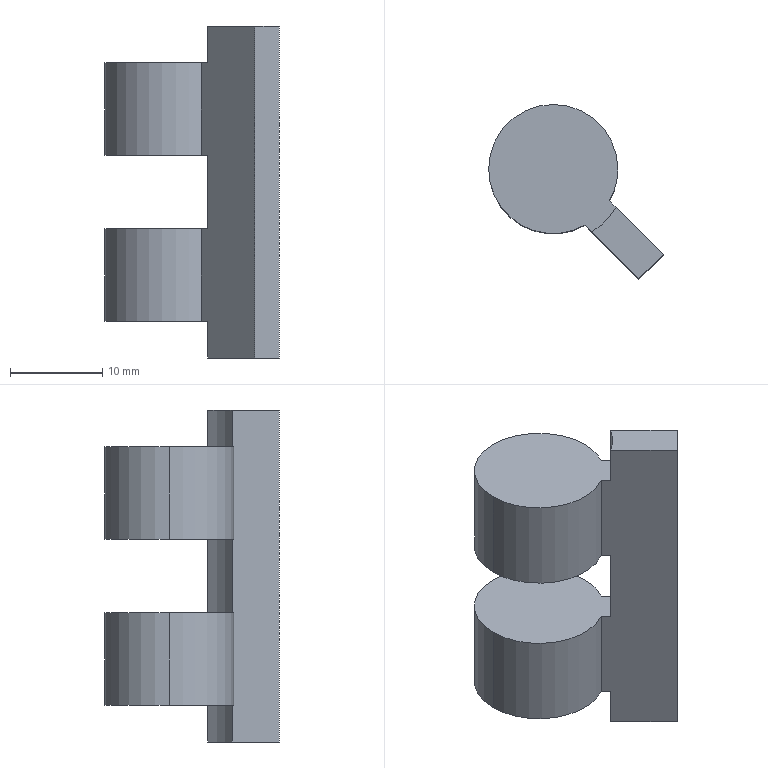Part | STEP file | 1 solid | 18 faces | box 18.932 x 18.932 x 36 mm | volume 4110 mm3 | cylinder 9 | plane 9 | commonest cylinder face diameters 14 x6 16 x3
STEP:
#1=CARTESIAN_POINT('',(0.,0.,0.));
#2=DIRECTION('',(0.,0.,1.));
#3=DIRECTION('',(1.,0.,0.));
#4=AXIS2_PLACEMENT_3D('',#1,#2,#3);
#5=CARTESIAN_POINT('',(-10.892,-5.625,-13.));
#6=VERTEX_POINT('',#5);
#7=CARTESIAN_POINT('',(-10.892,-5.625,-23.));
#8=VERTEX_POINT('',#7);
#9=CARTESIAN_POINT('',(-10.892,-5.625,-13.));
#10=DIRECTION('',(0.,0.,-1.));
#11=VECTOR('',#10,1.);
#12=LINE('',#9,#11);
#13=CARTESIAN_POINT('',(-3.892,-5.625,-23.));
#14=DIRECTION('',(0.,0.,1.));
#15=DIRECTION('',(-1.,0.,0.));
#16=AXIS2_PLACEMENT_3D('',#13,#14,#15);
#17=CYLINDRICAL_SURFACE('',#16,7.);
#18=CARTESIAN_POINT('',(6.283,10.));
#19=DIRECTION('',(0.,-1.));
#20=VECTOR('',#19,1.);
#21=LINE('',#18,#20);
#22=(GEOMETRIC_REPRESENTATION_CONTEXT(2)PARAMETRIC_REPRESENTATION_CONTEXT()REPRESENTATION_CONTEXT('',''));
#23=DEFINITIONAL_REPRESENTATION('',(#21),#22);
#24=PCURVE('',#17,#23);
#25=CARTESIAN_POINT('',(-3.892,-5.625,-23.));
#26=DIRECTION('',(0.,0.,1.));
#27=DIRECTION('',(-1.,0.,0.));
#28=AXIS2_PLACEMENT_3D('',#25,#26,#27);
#29=CYLINDRICAL_SURFACE('',#28,7.);
#30=CARTESIAN_POINT('',(0.,10.));
#31=DIRECTION('',(0.,-1.));
#32=VECTOR('',#31,1.);
#33=LINE('',#30,#32);
#34=(GEOMETRIC_REPRESENTATION_CONTEXT(2)PARAMETRIC_REPRESENTATION_CONTEXT()REPRESENTATION_CONTEXT('',''));
#35=DEFINITIONAL_REPRESENTATION('',(#33),#34);
#36=PCURVE('',#29,#35);
#37=SURFACE_CURVE('',#12,(#24,#36),.PCURVE_S1.);
#38=EDGE_CURVE('',#6,#8,#37,.T.);
#39=ORIENTED_EDGE('',*,*,#38,.F.);
#40=CARTESIAN_POINT('',(3.108,-5.625,-13.));
#41=VERTEX_POINT('',#40);
#42=CARTESIAN_POINT('',(-3.892,-5.625,-13.));
#43=DIRECTION('',(0.,0.,1.));
#44=DIRECTION('',(1.,0.,0.));
#45=AXIS2_PLACEMENT_3D('',#42,#43,#44);
#46=CIRCLE('',#45,7.);
#47=CARTESIAN_POINT('',(3.142,10.));
#48=DIRECTION('',(1.,0.));
#49=VECTOR('',#48,1.);
#50=LINE('',#47,#49);
#51=(GEOMETRIC_REPRESENTATION_CONTEXT(2)PARAMETRIC_REPRESENTATION_CONTEXT()REPRESENTATION_CONTEXT('',''));
#52=DEFINITIONAL_REPRESENTATION('',(#50),#51);
#53=PCURVE('',#17,#52);
#54=CARTESIAN_POINT('',(-3.892,-5.625,-13.));
#55=DIRECTION('',(0.,0.,1.));
#56=DIRECTION('',(-1.,0.,0.));
#57=AXIS2_PLACEMENT_3D('',#54,#55,#56);
#58=PLANE('',#57);
#59=CARTESIAN_POINT('',(0.,0.));
#60=DIRECTION('',(-1.,0.));
#61=AXIS2_PLACEMENT_2D('',#59,#60);
#62=CIRCLE('',#61,7.);
#63=(GEOMETRIC_REPRESENTATION_CONTEXT(2)PARAMETRIC_REPRESENTATION_CONTEXT()REPRESENTATION_CONTEXT('',''));
#64=DEFINITIONAL_REPRESENTATION('',(#62),#63);
#65=PCURVE('',#58,#64);
#66=SURFACE_CURVE('',#46,(#53,#65),.PCURVE_S1.);
#67=EDGE_CURVE('',#41,#6,#66,.T.);
#68=ORIENTED_EDGE('',*,*,#67,.F.);
#69=CARTESIAN_POINT('',(3.108,-5.625,-23.));
#70=VERTEX_POINT('',#69);
#71=CARTESIAN_POINT('',(3.108,-5.625,-13.));
#72=DIRECTION('',(0.,0.,-1.));
#73=VECTOR('',#72,1.);
#74=LINE('',#71,#73);
#75=CARTESIAN_POINT('',(3.142,10.));
#76=DIRECTION('',(0.,-1.));
#77=VECTOR('',#76,1.);
#78=LINE('',#75,#77);
#79=(GEOMETRIC_REPRESENTATION_CONTEXT(2)PARAMETRIC_REPRESENTATION_CONTEXT()REPRESENTATION_CONTEXT('',''));
#80=DEFINITIONAL_REPRESENTATION('',(#78),#79);
#81=PCURVE('',#17,#80);
#82=CARTESIAN_POINT('',(-3.892,-5.625,-23.));
#83=DIRECTION('',(0.,0.,1.));
#84=DIRECTION('',(-1.,0.,0.));
#85=AXIS2_PLACEMENT_3D('',#82,#83,#84);
#86=CYLINDRICAL_SURFACE('',#85,7.);
#87=CARTESIAN_POINT('',(3.142,10.));
#88=DIRECTION('',(0.,-1.));
#89=VECTOR('',#88,1.);
#90=LINE('',#87,#89);
#91=(GEOMETRIC_REPRESENTATION_CONTEXT(2)PARAMETRIC_REPRESENTATION_CONTEXT()REPRESENTATION_CONTEXT('',''));
#92=DEFINITIONAL_REPRESENTATION('',(#90),#91);
#93=PCURVE('',#86,#92);
#94=SURFACE_CURVE('',#74,(#81,#93),.PCURVE_S1.);
#95=EDGE_CURVE('',#41,#70,#94,.T.);
#96=ORIENTED_EDGE('',*,*,#95,.T.);
#97=CARTESIAN_POINT('',(-3.892,-5.625,-23.));
#98=DIRECTION('',(0.,0.,-1.));
#99=DIRECTION('',(-1.,0.,0.));
#100=AXIS2_PLACEMENT_3D('',#97,#98,#99);
#101=CIRCLE('',#100,7.);
#102=CARTESIAN_POINT('',(6.283,0.));
#103=DIRECTION('',(-1.,0.));
#104=VECTOR('',#103,1.);
#105=LINE('',#102,#104);
#106=(GEOMETRIC_REPRESENTATION_CONTEXT(2)PARAMETRIC_REPRESENTATION_CONTEXT()REPRESENTATION_CONTEXT('',''));
#107=DEFINITIONAL_REPRESENTATION('',(#105),#106);
#108=PCURVE('',#17,#107);
#109=CARTESIAN_POINT('',(-3.892,-5.625,-23.));
#110=DIRECTION('',(0.,0.,1.));
#111=DIRECTION('',(-1.,0.,0.));
#112=AXIS2_PLACEMENT_3D('',#109,#110,#111);
#113=PLANE('',#112);
#114=CARTESIAN_POINT('',(7.,0.));
#115=CARTESIAN_POINT('',(7.,-12.124));
#116=CARTESIAN_POINT('',(-3.5,-6.062));
#117=CARTESIAN_POINT('',(-14.,0.));
#118=CARTESIAN_POINT('',(-3.5,6.062));
#119=CARTESIAN_POINT('',(7.,12.124));
#120=CARTESIAN_POINT('',(7.,0.));
#121=(BOUNDED_CURVE()B_SPLINE_CURVE(2,(#114,#115,#116,#117,#118,#119,#120),.UNSPECIFIED.,.T.,.F.)B_SPLINE_CURVE_WITH_KNOTS((1,2,2,2,2,1),(-2.094,0.,2.094,4.189,6.283,8.378),.UNSPECIFIED.)CURVE()GEOMETRIC_REPRESENTATION_ITEM()RATIONAL_B_SPLINE_CURVE((1.,0.5,1.,0.5,1.,0.5,1.))REPRESENTATION_ITEM(''));
#122=(GEOMETRIC_REPRESENTATION_CONTEXT(2)PARAMETRIC_REPRESENTATION_CONTEXT()REPRESENTATION_CONTEXT('',''));
#123=DEFINITIONAL_REPRESENTATION('',(#121),#122);
#124=PCURVE('',#113,#123);
#125=SURFACE_CURVE('',#101,(#108,#124),.PCURVE_S1.);
#126=EDGE_CURVE('',#8,#70,#125,.T.);
#127=ORIENTED_EDGE('',*,*,#126,.F.);
#128=EDGE_LOOP('',(#39,#68,#96,#127));
#129=FACE_BOUND('',#128,.T.);
#130=ADVANCED_FACE('',(#129),#17,.T.);
#131=CARTESIAN_POINT('',(0.2816,-12.45,-23.));
#132=VERTEX_POINT('',#131);
#133=CARTESIAN_POINT('',(-0.4488,-11.72,-23.));
#134=VERTEX_POINT('',#133);
#135=CARTESIAN_POINT('',(0.2816,-12.45,-23.));
#136=DIRECTION('',(-0.7071,0.7071,0.));
#137=VECTOR('',#136,1.);
#138=LINE('',#135,#137);
#139=CARTESIAN_POINT('',(-4.173,6.825));
#140=DIRECTION('',(0.7071,-0.7071));
#141=VECTOR('',#140,1.);
#142=LINE('',#139,#141);
#143=(GEOMETRIC_REPRESENTATION_CONTEXT(2)PARAMETRIC_REPRESENTATION_CONTEXT()REPRESENTATION_CONTEXT('',''));
#144=DEFINITIONAL_REPRESENTATION('',(#142),#143);
#145=PCURVE('',#113,#144);
#146=CARTESIAN_POINT('',(-0.4488,-11.72,5.));
#147=DIRECTION('',(0.7071,0.7071,0.));
#148=DIRECTION('',(0.,0.,1.));
#149=AXIS2_PLACEMENT_3D('',#146,#147,#148);
#150=PLANE('',#149);
#151=CARTESIAN_POINT('',(-28.,1.033));
#152=DIRECTION('',(0.,-1.));
#153=VECTOR('',#152,1.);
#154=LINE('',#151,#153);
#155=(GEOMETRIC_REPRESENTATION_CONTEXT(2)PARAMETRIC_REPRESENTATION_CONTEXT()REPRESENTATION_CONTEXT('',''));
#156=DEFINITIONAL_REPRESENTATION('',(#154),#155);
#157=PCURVE('',#150,#156);
#158=SURFACE_CURVE('',#138,(#145,#157),.PCURVE_S1.);
#159=EDGE_CURVE('',#132,#134,#158,.T.);
#160=ORIENTED_EDGE('',*,*,#159,.F.);
#161=CARTESIAN_POINT('',(2.933,-9.798,-23.));
#162=VERTEX_POINT('',#161);
#163=CARTESIAN_POINT('',(-3.892,-5.625,-23.));
#164=DIRECTION('',(0.,0.,-1.));
#165=DIRECTION('',(0.8531,-0.5217,0.));
#166=AXIS2_PLACEMENT_3D('',#163,#164,#165);
#167=CIRCLE('',#166,8.);
#168=CARTESIAN_POINT('',(-6.825,4.173));
#169=CARTESIAN_POINT('',(0.4035,15.995));
#170=CARTESIAN_POINT('',(7.027,3.824));
#171=CARTESIAN_POINT('',(13.65,-8.347));
#172=CARTESIAN_POINT('',(-0.2018,-7.997));
#173=CARTESIAN_POINT('',(-14.054,-7.648));
#174=CARTESIAN_POINT('',(-6.825,4.173));
#175=(BOUNDED_CURVE()B_SPLINE_CURVE(2,(#168,#169,#170,#171,#172,#173,#174),.UNSPECIFIED.,.T.,.F.)B_SPLINE_CURVE_WITH_KNOTS((1,2,2,2,2,1),(-2.094,0.,2.094,4.189,6.283,8.378),.UNSPECIFIED.)CURVE()GEOMETRIC_REPRESENTATION_ITEM()RATIONAL_B_SPLINE_CURVE((1.,0.5,1.,0.5,1.,0.5,1.))REPRESENTATION_ITEM(''));
#176=(GEOMETRIC_REPRESENTATION_CONTEXT(2)PARAMETRIC_REPRESENTATION_CONTEXT()REPRESENTATION_CONTEXT('',''));
#177=DEFINITIONAL_REPRESENTATION('',(#175),#176);
#178=PCURVE('',#113,#177);
#179=CARTESIAN_POINT('',(-3.892,-5.625,-37.973));
#180=DIRECTION('',(0.,0.,1.));
#181=DIRECTION('',(-1.,0.,0.));
#182=AXIS2_PLACEMENT_3D('',#179,#180,#181);
#183=CYLINDRICAL_SURFACE('',#182,8.);
#184=CARTESIAN_POINT('',(2.593,14.973));
#185=DIRECTION('',(-1.,0.));
#186=VECTOR('',#185,1.);
#187=LINE('',#184,#186);
#188=(GEOMETRIC_REPRESENTATION_CONTEXT(2)PARAMETRIC_REPRESENTATION_CONTEXT()REPRESENTATION_CONTEXT('',''));
#189=DEFINITIONAL_REPRESENTATION('',(#187),#188);
#190=PCURVE('',#183,#189);
#191=SURFACE_CURVE('',#167,(#178,#190),.PCURVE_S1.);
#192=EDGE_CURVE('',#162,#132,#191,.T.);
#193=ORIENTED_EDGE('',*,*,#192,.F.);
#194=CARTESIAN_POINT('',(2.203,-9.068,-23.));
#195=VERTEX_POINT('',#194);
#196=CARTESIAN_POINT('',(2.203,-9.068,-23.));
#197=DIRECTION('',(0.7071,-0.7071,0.));
#198=VECTOR('',#197,1.);
#199=LINE('',#196,#198);
#200=CARTESIAN_POINT('',(-6.095,3.443));
#201=DIRECTION('',(-0.7071,0.7071));
#202=VECTOR('',#201,1.);
#203=LINE('',#200,#202);
#204=(GEOMETRIC_REPRESENTATION_CONTEXT(2)PARAMETRIC_REPRESENTATION_CONTEXT()REPRESENTATION_CONTEXT('',''));
#205=DEFINITIONAL_REPRESENTATION('',(#203),#204);
#206=PCURVE('',#113,#205);
#207=CARTESIAN_POINT('',(8.041,-14.906,5.));
#208=DIRECTION('',(-0.7071,-0.7071,0.));
#209=DIRECTION('',(0.7071,-0.7071,0.));
#210=AXIS2_PLACEMENT_3D('',#207,#208,#209);
#211=PLANE('',#210);
#212=CARTESIAN_POINT('',(-8.256,-28.));
#213=DIRECTION('',(1.,0.));
#214=VECTOR('',#213,1.);
#215=LINE('',#212,#214);
#216=(GEOMETRIC_REPRESENTATION_CONTEXT(2)PARAMETRIC_REPRESENTATION_CONTEXT()REPRESENTATION_CONTEXT('',''));
#217=DEFINITIONAL_REPRESENTATION('',(#215),#216);
#218=PCURVE('',#211,#217);
#219=SURFACE_CURVE('',#199,(#206,#218),.PCURVE_S1.);
#220=EDGE_CURVE('',#195,#162,#219,.T.);
#221=ORIENTED_EDGE('',*,*,#220,.F.);
#222=CARTESIAN_POINT('',(-3.892,-5.625,-23.));
#223=DIRECTION('',(0.,0.,-1.));
#224=DIRECTION('',(1.,0.,0.));
#225=AXIS2_PLACEMENT_3D('',#222,#223,#224);
#226=CIRCLE('',#225,7.);
#227=CARTESIAN_POINT('',(-7.,0.));
#228=CARTESIAN_POINT('',(-7.,12.124));
#229=CARTESIAN_POINT('',(3.5,6.062));
#230=CARTESIAN_POINT('',(14.,0.));
#231=CARTESIAN_POINT('',(3.5,-6.062));
#232=CARTESIAN_POINT('',(-7.,-12.124));
#233=CARTESIAN_POINT('',(-7.,0.));
#234=(BOUNDED_CURVE()B_SPLINE_CURVE(2,(#227,#228,#229,#230,#231,#232,#233),.UNSPECIFIED.,.T.,.F.)B_SPLINE_CURVE_WITH_KNOTS((1,2,2,2,2,1),(-2.094,0.,2.094,4.189,6.283,8.378),.UNSPECIFIED.)CURVE()GEOMETRIC_REPRESENTATION_ITEM()RATIONAL_B_SPLINE_CURVE((1.,0.5,1.,0.5,1.,0.5,1.))REPRESENTATION_ITEM(''));
#235=(GEOMETRIC_REPRESENTATION_CONTEXT(2)PARAMETRIC_REPRESENTATION_CONTEXT()REPRESENTATION_CONTEXT('',''));
#236=DEFINITIONAL_REPRESENTATION('',(#234),#235);
#237=PCURVE('',#113,#236);
#238=CARTESIAN_POINT('',(3.142,0.));
#239=DIRECTION('',(-1.,0.));
#240=VECTOR('',#239,1.);
#241=LINE('',#238,#240);
#242=(GEOMETRIC_REPRESENTATION_CONTEXT(2)PARAMETRIC_REPRESENTATION_CONTEXT()REPRESENTATION_CONTEXT('',''));
#243=DEFINITIONAL_REPRESENTATION('',(#241),#242);
#244=PCURVE('',#86,#243);
#245=SURFACE_CURVE('',#226,(#237,#244),.PCURVE_S1.);
#246=EDGE_CURVE('',#70,#195,#245,.T.);
#247=ORIENTED_EDGE('',*,*,#246,.F.);
#248=ORIENTED_EDGE('',*,*,#126,.F.);
#249=CARTESIAN_POINT('',(-3.892,-5.625,-23.));
#250=DIRECTION('',(0.,0.,-1.));
#251=DIRECTION('',(0.4919,-0.8707,0.));
#252=AXIS2_PLACEMENT_3D('',#249,#250,#251);
#253=CIRCLE('',#252,7.);
#254=CARTESIAN_POINT('',(-3.443,6.095));
#255=CARTESIAN_POINT('',(7.113,12.058));
#256=CARTESIAN_POINT('',(7.,-0.06558));
#257=CARTESIAN_POINT('',(6.886,-12.189));
#258=CARTESIAN_POINT('',(-3.557,-6.029));
#259=CARTESIAN_POINT('',(-13.999,0.1312));
#260=CARTESIAN_POINT('',(-3.443,6.095));
#261=(BOUNDED_CURVE()B_SPLINE_CURVE(2,(#254,#255,#256,#257,#258,#259,#260),.UNSPECIFIED.,.T.,.F.)B_SPLINE_CURVE_WITH_KNOTS((1,2,2,2,2,1),(-2.094,0.,2.094,4.189,6.283,8.378),.UNSPECIFIED.)CURVE()GEOMETRIC_REPRESENTATION_ITEM()RATIONAL_B_SPLINE_CURVE((1.,0.5,1.,0.5,1.,0.5,1.))REPRESENTATION_ITEM(''));
#262=(GEOMETRIC_REPRESENTATION_CONTEXT(2)PARAMETRIC_REPRESENTATION_CONTEXT()REPRESENTATION_CONTEXT('',''));
#263=DEFINITIONAL_REPRESENTATION('',(#261),#262);
#264=PCURVE('',#113,#263);
#265=CARTESIAN_POINT('',(2.085,0.));
#266=DIRECTION('',(-1.,0.));
#267=VECTOR('',#266,1.);
#268=LINE('',#265,#267);
#269=(GEOMETRIC_REPRESENTATION_CONTEXT(2)PARAMETRIC_REPRESENTATION_CONTEXT()REPRESENTATION_CONTEXT('',''));
#270=DEFINITIONAL_REPRESENTATION('',(#268),#269);
#271=PCURVE('',#29,#270);
#272=SURFACE_CURVE('',#253,(#264,#271),.PCURVE_S1.);
#273=EDGE_CURVE('',#134,#8,#272,.T.);
#274=ORIENTED_EDGE('',*,*,#273,.F.);
#275=EDGE_LOOP('',(#160,#193,#221,#247,#248,#274));
#276=FACE_BOUND('',#275,.F.);
#277=ADVANCED_FACE('',(#276),#113,.F.);
#278=CARTESIAN_POINT('',(-0.4488,-11.72,-13.));
#279=VERTEX_POINT('',#278);
#280=CARTESIAN_POINT('',(0.2816,-12.45,-13.));
#281=VERTEX_POINT('',#280);
#282=CARTESIAN_POINT('',(-0.4488,-11.72,-13.));
#283=DIRECTION('',(0.7071,-0.7071,0.));
#284=VECTOR('',#283,1.);
#285=LINE('',#282,#284);
#286=CARTESIAN_POINT('',(-18.,0.));
#287=DIRECTION('',(0.,1.));
#288=VECTOR('',#287,1.);
#289=LINE('',#286,#288);
#290=(GEOMETRIC_REPRESENTATION_CONTEXT(2)PARAMETRIC_REPRESENTATION_CONTEXT()REPRESENTATION_CONTEXT('',''));
#291=DEFINITIONAL_REPRESENTATION('',(#289),#290);
#292=PCURVE('',#150,#291);
#293=CARTESIAN_POINT('',(-3.443,6.095));
#294=DIRECTION('',(-0.7071,0.7071));
#295=VECTOR('',#294,1.);
#296=LINE('',#293,#295);
#297=(GEOMETRIC_REPRESENTATION_CONTEXT(2)PARAMETRIC_REPRESENTATION_CONTEXT()REPRESENTATION_CONTEXT('',''));
#298=DEFINITIONAL_REPRESENTATION('',(#296),#297);
#299=PCURVE('',#58,#298);
#300=SURFACE_CURVE('',#285,(#292,#299),.PCURVE_S1.);
#301=EDGE_CURVE('',#279,#281,#300,.T.);
#302=ORIENTED_EDGE('',*,*,#301,.T.);
#303=CARTESIAN_POINT('',(0.2816,-12.45,-5.));
#304=VERTEX_POINT('',#303);
#305=CARTESIAN_POINT('',(0.2816,-12.45,-13.));
#306=DIRECTION('',(0.,0.,1.));
#307=VECTOR('',#306,1.);
#308=LINE('',#305,#307);
#309=CARTESIAN_POINT('',(-18.,1.033));
#310=DIRECTION('',(1.,0.));
#311=VECTOR('',#310,1.);
#312=LINE('',#309,#311);
#313=(GEOMETRIC_REPRESENTATION_CONTEXT(2)PARAMETRIC_REPRESENTATION_CONTEXT()REPRESENTATION_CONTEXT('',''));
#314=DEFINITIONAL_REPRESENTATION('',(#312),#313);
#315=PCURVE('',#150,#314);
#316=CARTESIAN_POINT('',(-3.892,-5.625,-37.973));
#317=DIRECTION('',(0.,0.,1.));
#318=DIRECTION('',(-1.,0.,0.));
#319=AXIS2_PLACEMENT_3D('',#316,#317,#318);
#320=CYLINDRICAL_SURFACE('',#319,8.);
#321=CARTESIAN_POINT('',(2.12,24.973));
#322=DIRECTION('',(0.,1.));
#323=VECTOR('',#322,1.);
#324=LINE('',#321,#323);
#325=(GEOMETRIC_REPRESENTATION_CONTEXT(2)PARAMETRIC_REPRESENTATION_CONTEXT()REPRESENTATION_CONTEXT('',''));
#326=DEFINITIONAL_REPRESENTATION('',(#324),#325);
#327=PCURVE('',#320,#326);
#328=SURFACE_CURVE('',#308,(#315,#327),.PCURVE_S1.);
#329=EDGE_CURVE('',#281,#304,#328,.T.);
#330=ORIENTED_EDGE('',*,*,#329,.T.);
#331=CARTESIAN_POINT('',(-0.4488,-11.72,-5.));
#332=VERTEX_POINT('',#331);
#333=CARTESIAN_POINT('',(0.2816,-12.45,-5.));
#334=DIRECTION('',(-0.7071,0.7071,0.));
#335=VECTOR('',#334,1.);
#336=LINE('',#333,#335);
#337=CARTESIAN_POINT('',(-10.,1.033));
#338=DIRECTION('',(0.,-1.));
#339=VECTOR('',#338,1.);
#340=LINE('',#337,#339);
#341=(GEOMETRIC_REPRESENTATION_CONTEXT(2)PARAMETRIC_REPRESENTATION_CONTEXT()REPRESENTATION_CONTEXT('',''));
#342=DEFINITIONAL_REPRESENTATION('',(#340),#341);
#343=PCURVE('',#150,#342);
#344=CARTESIAN_POINT('',(-3.892,-5.625,-5.));
#345=DIRECTION('',(0.,0.,-1.));
#346=DIRECTION('',(0.,1.,0.));
#347=AXIS2_PLACEMENT_3D('',#344,#345,#346);
#348=PLANE('',#347);
#349=CARTESIAN_POINT('',(-6.825,4.173));
#350=DIRECTION('',(0.7071,-0.7071));
#351=VECTOR('',#350,1.);
#352=LINE('',#349,#351);
#353=(GEOMETRIC_REPRESENTATION_CONTEXT(2)PARAMETRIC_REPRESENTATION_CONTEXT()REPRESENTATION_CONTEXT('',''));
#354=DEFINITIONAL_REPRESENTATION('',(#352),#353);
#355=PCURVE('',#348,#354);
#356=SURFACE_CURVE('',#336,(#343,#355),.PCURVE_S1.);
#357=EDGE_CURVE('',#304,#332,#356,.T.);
#358=ORIENTED_EDGE('',*,*,#357,.T.);
#359=CARTESIAN_POINT('',(-0.4488,-11.72,5.));
#360=VERTEX_POINT('',#359);
#361=CARTESIAN_POINT('',(-0.4488,-11.72,-5.));
#362=DIRECTION('',(0.,0.,1.));
#363=VECTOR('',#362,1.);
#364=LINE('',#361,#363);
#365=CARTESIAN_POINT('',(-10.,0.));
#366=DIRECTION('',(1.,0.));
#367=VECTOR('',#366,1.);
#368=LINE('',#365,#367);
#369=(GEOMETRIC_REPRESENTATION_CONTEXT(2)PARAMETRIC_REPRESENTATION_CONTEXT()REPRESENTATION_CONTEXT('',''));
#370=DEFINITIONAL_REPRESENTATION('',(#368),#369);
#371=PCURVE('',#150,#370);
#372=CARTESIAN_POINT('',(-3.892,-5.625,5.));
#373=DIRECTION('',(0.,0.,-1.));
#374=DIRECTION('',(1.,0.,0.));
#375=AXIS2_PLACEMENT_3D('',#372,#373,#374);
#376=CYLINDRICAL_SURFACE('',#375,7.);
#377=CARTESIAN_POINT('',(1.057,10.));
#378=DIRECTION('',(0.,-1.));
#379=VECTOR('',#378,1.);
#380=LINE('',#377,#379);
#381=(GEOMETRIC_REPRESENTATION_CONTEXT(2)PARAMETRIC_REPRESENTATION_CONTEXT()REPRESENTATION_CONTEXT('',''));
#382=DEFINITIONAL_REPRESENTATION('',(#380),#381);
#383=PCURVE('',#376,#382);
#384=SURFACE_CURVE('',#364,(#371,#383),.PCURVE_S1.);
#385=EDGE_CURVE('',#332,#360,#384,.T.);
#386=ORIENTED_EDGE('',*,*,#385,.T.);
#387=CARTESIAN_POINT('',(0.2816,-12.45,5.));
#388=VERTEX_POINT('',#387);
#389=CARTESIAN_POINT('',(-0.4488,-11.72,5.));
#390=DIRECTION('',(0.7071,-0.7071,0.));
#391=VECTOR('',#390,1.);
#392=LINE('',#389,#391);
#393=CARTESIAN_POINT('',(0.,0.));
#394=DIRECTION('',(0.,1.));
#395=VECTOR('',#394,1.);
#396=LINE('',#393,#395);
#397=(GEOMETRIC_REPRESENTATION_CONTEXT(2)PARAMETRIC_REPRESENTATION_CONTEXT()REPRESENTATION_CONTEXT('',''));
#398=DEFINITIONAL_REPRESENTATION('',(#396),#397);
#399=PCURVE('',#150,#398);
#400=CARTESIAN_POINT('',(-3.892,-5.625,5.));
#401=DIRECTION('',(0.,0.,-1.));
#402=DIRECTION('',(0.,1.,0.));
#403=AXIS2_PLACEMENT_3D('',#400,#401,#402);
#404=PLANE('',#403);
#405=CARTESIAN_POINT('',(-6.095,3.443));
#406=DIRECTION('',(-0.7071,0.7071));
#407=VECTOR('',#406,1.);
#408=LINE('',#405,#407);
#409=(GEOMETRIC_REPRESENTATION_CONTEXT(2)PARAMETRIC_REPRESENTATION_CONTEXT()REPRESENTATION_CONTEXT('',''));
#410=DEFINITIONAL_REPRESENTATION('',(#408),#409);
#411=PCURVE('',#404,#410);
#412=SURFACE_CURVE('',#392,(#399,#411),.PCURVE_S1.);
#413=EDGE_CURVE('',#360,#388,#412,.T.);
#414=ORIENTED_EDGE('',*,*,#413,.T.);
#415=CARTESIAN_POINT('',(0.2816,-12.45,9.));
#416=VERTEX_POINT('',#415);
#417=CARTESIAN_POINT('',(0.2816,-12.45,5.));
#418=DIRECTION('',(0.,0.,1.));
#419=VECTOR('',#418,1.);
#420=LINE('',#417,#419);
#421=CARTESIAN_POINT('',(0.,1.033));
#422=DIRECTION('',(1.,0.));
#423=VECTOR('',#422,1.);
#424=LINE('',#421,#423);
#425=(GEOMETRIC_REPRESENTATION_CONTEXT(2)PARAMETRIC_REPRESENTATION_CONTEXT()REPRESENTATION_CONTEXT('',''));
#426=DEFINITIONAL_REPRESENTATION('',(#424),#425);
#427=PCURVE('',#150,#426);
#428=CARTESIAN_POINT('',(-3.892,-5.625,-37.973));
#429=DIRECTION('',(0.,0.,1.));
#430=DIRECTION('',(-1.,0.,0.));
#431=AXIS2_PLACEMENT_3D('',#428,#429,#430);
#432=CYLINDRICAL_SURFACE('',#431,8.);
#433=CARTESIAN_POINT('',(2.12,42.973));
#434=DIRECTION('',(0.,1.));
#435=VECTOR('',#434,1.);
#436=LINE('',#433,#435);
#437=(GEOMETRIC_REPRESENTATION_CONTEXT(2)PARAMETRIC_REPRESENTATION_CONTEXT()REPRESENTATION_CONTEXT('',''));
#438=DEFINITIONAL_REPRESENTATION('',(#436),#437);
#439=PCURVE('',#432,#438);
#440=SURFACE_CURVE('',#420,(#427,#439),.PCURVE_S1.);
#441=EDGE_CURVE('',#388,#416,#440,.T.);
#442=ORIENTED_EDGE('',*,*,#441,.T.);
#443=CARTESIAN_POINT('',(5.389,-17.557,9.));
#444=VERTEX_POINT('',#443);
#445=CARTESIAN_POINT('',(0.2816,-12.45,9.));
#446=DIRECTION('',(0.7071,-0.7071,0.));
#447=VECTOR('',#446,1.);
#448=LINE('',#445,#447);
#449=CARTESIAN_POINT('',(4.,1.033));
#450=DIRECTION('',(0.,1.));
#451=VECTOR('',#450,1.);
#452=LINE('',#449,#451);
#453=(GEOMETRIC_REPRESENTATION_CONTEXT(2)PARAMETRIC_REPRESENTATION_CONTEXT()REPRESENTATION_CONTEXT('',''));
#454=DEFINITIONAL_REPRESENTATION('',(#452),#453);
#455=PCURVE('',#150,#454);
#456=CARTESIAN_POINT('',(-3.892,-5.625,9.));
#457=DIRECTION('',(0.,0.,1.));
#458=DIRECTION('',(-1.,0.,0.));
#459=AXIS2_PLACEMENT_3D('',#456,#457,#458);
#460=PLANE('',#459);
#461=CARTESIAN_POINT('',(-4.173,6.825));
#462=DIRECTION('',(-0.7071,0.7071));
#463=VECTOR('',#462,1.);
#464=LINE('',#461,#463);
#465=(GEOMETRIC_REPRESENTATION_CONTEXT(2)PARAMETRIC_REPRESENTATION_CONTEXT()REPRESENTATION_CONTEXT('',''));
#466=DEFINITIONAL_REPRESENTATION('',(#464),#465);
#467=PCURVE('',#460,#466);
#468=SURFACE_CURVE('',#448,(#455,#467),.PCURVE_S1.);
#469=EDGE_CURVE('',#416,#444,#468,.T.);
#470=ORIENTED_EDGE('',*,*,#469,.T.);
#471=CARTESIAN_POINT('',(5.389,-17.557,-27.));
#472=VERTEX_POINT('',#471);
#473=CARTESIAN_POINT('',(5.389,-17.557,-27.));
#474=DIRECTION('',(0.,0.,1.));
#475=VECTOR('',#474,1.);
#476=LINE('',#473,#475);
#477=CARTESIAN_POINT('',(-32.,8.256));
#478=DIRECTION('',(1.,0.));
#479=VECTOR('',#478,1.);
#480=LINE('',#477,#479);
#481=(GEOMETRIC_REPRESENTATION_CONTEXT(2)PARAMETRIC_REPRESENTATION_CONTEXT()REPRESENTATION_CONTEXT('',''));
#482=DEFINITIONAL_REPRESENTATION('',(#480),#481);
#483=PCURVE('',#150,#482);
#484=CARTESIAN_POINT('',(5.389,-17.557,5.));
#485=DIRECTION('',(-0.7071,0.7071,0.));
#486=DIRECTION('',(0.,0.,-1.));
#487=AXIS2_PLACEMENT_3D('',#484,#485,#486);
#488=PLANE('',#487);
#489=CARTESIAN_POINT('',(32.,0.));
#490=DIRECTION('',(-1.,0.));
#491=VECTOR('',#490,1.);
#492=LINE('',#489,#491);
#493=(GEOMETRIC_REPRESENTATION_CONTEXT(2)PARAMETRIC_REPRESENTATION_CONTEXT()REPRESENTATION_CONTEXT('',''));
#494=DEFINITIONAL_REPRESENTATION('',(#492),#493);
#495=PCURVE('',#488,#494);
#496=SURFACE_CURVE('',#476,(#483,#495),.PCURVE_S1.);
#497=EDGE_CURVE('',#472,#444,#496,.T.);
#498=ORIENTED_EDGE('',*,*,#497,.F.);
#499=CARTESIAN_POINT('',(0.2816,-12.45,-27.));
#500=VERTEX_POINT('',#499);
#501=CARTESIAN_POINT('',(5.389,-17.557,-27.));
#502=DIRECTION('',(-0.7071,0.7071,0.));
#503=VECTOR('',#502,1.);
#504=LINE('',#501,#503);
#505=CARTESIAN_POINT('',(-32.,8.256));
#506=DIRECTION('',(0.,-1.));
#507=VECTOR('',#506,1.);
#508=LINE('',#505,#507);
#509=(GEOMETRIC_REPRESENTATION_CONTEXT(2)PARAMETRIC_REPRESENTATION_CONTEXT()REPRESENTATION_CONTEXT('',''));
#510=DEFINITIONAL_REPRESENTATION('',(#508),#509);
#511=PCURVE('',#150,#510);
#512=CARTESIAN_POINT('',(-20.459,-42.,-27.));
#513=DIRECTION('',(0.,0.,-1.));
#514=DIRECTION('',(0.,1.,0.));
#515=AXIS2_PLACEMENT_3D('',#512,#513,#514);
#516=PLANE('',#515);
#517=CARTESIAN_POINT('',(24.443,25.848));
#518=DIRECTION('',(0.7071,-0.7071));
#519=VECTOR('',#518,1.);
#520=LINE('',#517,#519);
#521=(GEOMETRIC_REPRESENTATION_CONTEXT(2)PARAMETRIC_REPRESENTATION_CONTEXT()REPRESENTATION_CONTEXT('',''));
#522=DEFINITIONAL_REPRESENTATION('',(#520),#521);
#523=PCURVE('',#516,#522);
#524=SURFACE_CURVE('',#504,(#511,#523),.PCURVE_S1.);
#525=EDGE_CURVE('',#472,#500,#524,.T.);
#526=ORIENTED_EDGE('',*,*,#525,.T.);
#527=CARTESIAN_POINT('',(0.2816,-12.45,-27.));
#528=DIRECTION('',(0.,0.,1.));
#529=VECTOR('',#528,1.);
#530=LINE('',#527,#529);
#531=CARTESIAN_POINT('',(-32.,1.033));
#532=DIRECTION('',(1.,0.));
#533=VECTOR('',#532,1.);
#534=LINE('',#531,#533);
#535=(GEOMETRIC_REPRESENTATION_CONTEXT(2)PARAMETRIC_REPRESENTATION_CONTEXT()REPRESENTATION_CONTEXT('',''));
#536=DEFINITIONAL_REPRESENTATION('',(#534),#535);
#537=PCURVE('',#150,#536);
#538=CARTESIAN_POINT('',(2.12,10.973));
#539=DIRECTION('',(0.,1.));
#540=VECTOR('',#539,1.);
#541=LINE('',#538,#540);
#542=(GEOMETRIC_REPRESENTATION_CONTEXT(2)PARAMETRIC_REPRESENTATION_CONTEXT()REPRESENTATION_CONTEXT('',''));
#543=DEFINITIONAL_REPRESENTATION('',(#541),#542);
#544=PCURVE('',#183,#543);
#545=SURFACE_CURVE('',#530,(#537,#544),.PCURVE_S1.);
#546=EDGE_CURVE('',#500,#132,#545,.T.);
#547=ORIENTED_EDGE('',*,*,#546,.T.);
#548=ORIENTED_EDGE('',*,*,#159,.T.);
#549=CARTESIAN_POINT('',(-0.4488,-11.72,-23.));
#550=DIRECTION('',(0.,0.,1.));
#551=VECTOR('',#550,1.);
#552=LINE('',#549,#551);
#553=CARTESIAN_POINT('',(-28.,0.));
#554=DIRECTION('',(1.,0.));
#555=VECTOR('',#554,1.);
#556=LINE('',#553,#555);
#557=(GEOMETRIC_REPRESENTATION_CONTEXT(2)PARAMETRIC_REPRESENTATION_CONTEXT()REPRESENTATION_CONTEXT('',''));
#558=DEFINITIONAL_REPRESENTATION('',(#556),#557);
#559=PCURVE('',#150,#558);
#560=CARTESIAN_POINT('',(2.085,0.));
#561=DIRECTION('',(0.,1.));
#562=VECTOR('',#561,1.);
#563=LINE('',#560,#562);
#564=(GEOMETRIC_REPRESENTATION_CONTEXT(2)PARAMETRIC_REPRESENTATION_CONTEXT()REPRESENTATION_CONTEXT('',''));
#565=DEFINITIONAL_REPRESENTATION('',(#563),#564);
#566=PCURVE('',#29,#565);
#567=SURFACE_CURVE('',#552,(#559,#566),.PCURVE_S1.);
#568=EDGE_CURVE('',#134,#279,#567,.T.);
#569=ORIENTED_EDGE('',*,*,#568,.T.);
#570=EDGE_LOOP('',(#302,#330,#358,#386,#414,#442,#470,#498,#526,#547,#548,#569));
#571=FACE_BOUND('',#570,.F.);
#572=ADVANCED_FACE('',(#571),#150,.F.);
#573=CARTESIAN_POINT('',(2.933,-9.798,-13.));
#574=VERTEX_POINT('',#573);
#575=CARTESIAN_POINT('',(2.203,-9.068,-13.));
#576=VERTEX_POINT('',#575);
#577=CARTESIAN_POINT('',(2.933,-9.798,-13.));
#578=DIRECTION('',(-0.7071,0.7071,0.));
#579=VECTOR('',#578,1.);
#580=LINE('',#577,#579);
#581=CARTESIAN_POINT('',(-6.825,4.173));
#582=DIRECTION('',(0.7071,-0.7071));
#583=VECTOR('',#582,1.);
#584=LINE('',#581,#583);
#585=(GEOMETRIC_REPRESENTATION_CONTEXT(2)PARAMETRIC_REPRESENTATION_CONTEXT()REPRESENTATION_CONTEXT('',''));
#586=DEFINITIONAL_REPRESENTATION('',(#584),#585);
#587=PCURVE('',#58,#586);
#588=CARTESIAN_POINT('',(-7.223,-18.));
#589=DIRECTION('',(-1.,0.));
#590=VECTOR('',#589,1.);
#591=LINE('',#588,#590);
#592=(GEOMETRIC_REPRESENTATION_CONTEXT(2)PARAMETRIC_REPRESENTATION_CONTEXT()REPRESENTATION_CONTEXT('',''));
#593=DEFINITIONAL_REPRESENTATION('',(#591),#592);
#594=PCURVE('',#211,#593);
#595=SURFACE_CURVE('',#580,(#587,#594),.PCURVE_S1.);
#596=EDGE_CURVE('',#574,#576,#595,.T.);
#597=ORIENTED_EDGE('',*,*,#596,.F.);
#598=CARTESIAN_POINT('',(-3.892,-5.625,-13.));
#599=DIRECTION('',(0.,0.,1.));
#600=DIRECTION('',(0.5217,-0.8531,0.));
#601=AXIS2_PLACEMENT_3D('',#598,#599,#600);
#602=CIRCLE('',#601,8.);
#603=CARTESIAN_POINT('',(0.,0.));
#604=DIRECTION('',(-0.5217,0.8531));
#605=AXIS2_PLACEMENT_2D('',#603,#604);
#606=CIRCLE('',#605,8.);
#607=(GEOMETRIC_REPRESENTATION_CONTEXT(2)PARAMETRIC_REPRESENTATION_CONTEXT()REPRESENTATION_CONTEXT('',''));
#608=DEFINITIONAL_REPRESENTATION('',(#606),#607);
#609=PCURVE('',#58,#608);
#610=CARTESIAN_POINT('',(2.12,24.973));
#611=DIRECTION('',(1.,0.));
#612=VECTOR('',#611,1.);
#613=LINE('',#610,#612);
#614=(GEOMETRIC_REPRESENTATION_CONTEXT(2)PARAMETRIC_REPRESENTATION_CONTEXT()REPRESENTATION_CONTEXT('',''));
#615=DEFINITIONAL_REPRESENTATION('',(#613),#614);
#616=PCURVE('',#320,#615);
#617=SURFACE_CURVE('',#602,(#609,#616),.PCURVE_S1.);
#618=EDGE_CURVE('',#281,#574,#617,.T.);
#619=ORIENTED_EDGE('',*,*,#618,.F.);
#620=ORIENTED_EDGE('',*,*,#301,.F.);
#621=CARTESIAN_POINT('',(-3.892,-5.625,-13.));
#622=DIRECTION('',(0.,0.,1.));
#623=DIRECTION('',(-1.,0.,0.));
#624=AXIS2_PLACEMENT_3D('',#621,#622,#623);
#625=CIRCLE('',#624,7.);
#626=CARTESIAN_POINT('',(0.,0.));
#627=DIRECTION('',(1.,0.));
#628=AXIS2_PLACEMENT_2D('',#626,#627);
#629=CIRCLE('',#628,7.);
#630=(GEOMETRIC_REPRESENTATION_CONTEXT(2)PARAMETRIC_REPRESENTATION_CONTEXT()REPRESENTATION_CONTEXT('',''));
#631=DEFINITIONAL_REPRESENTATION('',(#629),#630);
#632=PCURVE('',#58,#631);
#633=CARTESIAN_POINT('',(0.,10.));
#634=DIRECTION('',(1.,0.));
#635=VECTOR('',#634,1.);
#636=LINE('',#633,#635);
#637=(GEOMETRIC_REPRESENTATION_CONTEXT(2)PARAMETRIC_REPRESENTATION_CONTEXT()REPRESENTATION_CONTEXT('',''));
#638=DEFINITIONAL_REPRESENTATION('',(#636),#637);
#639=PCURVE('',#29,#638);
#640=SURFACE_CURVE('',#625,(#632,#639),.PCURVE_S1.);
#641=EDGE_CURVE('',#6,#279,#640,.T.);
#642=ORIENTED_EDGE('',*,*,#641,.F.);
#643=ORIENTED_EDGE('',*,*,#67,.F.);
#644=CARTESIAN_POINT('',(-3.892,-5.625,-13.));
#645=DIRECTION('',(0.,0.,1.));
#646=DIRECTION('',(0.8707,-0.4919,0.));
#647=AXIS2_PLACEMENT_3D('',#644,#645,#646);
#648=CIRCLE('',#647,7.);
#649=CARTESIAN_POINT('',(0.,0.));
#650=DIRECTION('',(-0.8707,0.4919));
#651=AXIS2_PLACEMENT_2D('',#649,#650);
#652=CIRCLE('',#651,7.);
#653=(GEOMETRIC_REPRESENTATION_CONTEXT(2)PARAMETRIC_REPRESENTATION_CONTEXT()REPRESENTATION_CONTEXT('',''));
#654=DEFINITIONAL_REPRESENTATION('',(#652),#653);
#655=PCURVE('',#58,#654);
#656=CARTESIAN_POINT('',(2.627,10.));
#657=DIRECTION('',(1.,0.));
#658=VECTOR('',#657,1.);
#659=LINE('',#656,#658);
#660=(GEOMETRIC_REPRESENTATION_CONTEXT(2)PARAMETRIC_REPRESENTATION_CONTEXT()REPRESENTATION_CONTEXT('',''));
#661=DEFINITIONAL_REPRESENTATION('',(#659),#660);
#662=PCURVE('',#86,#661);
#663=SURFACE_CURVE('',#648,(#655,#662),.PCURVE_S1.);
#664=EDGE_CURVE('',#576,#41,#663,.T.);
#665=ORIENTED_EDGE('',*,*,#664,.F.);
#666=EDGE_LOOP('',(#597,#619,#620,#642,#643,#665));
#667=FACE_BOUND('',#666,.F.);
#668=ADVANCED_FACE('',(#667),#58,.T.);
#669=CARTESIAN_POINT('',(2.933,-9.798,-27.));
#670=VERTEX_POINT('',#669);
#671=CARTESIAN_POINT('',(8.041,-14.906,-27.));
#672=VERTEX_POINT('',#671);
#673=CARTESIAN_POINT('',(2.933,-9.798,-27.));
#674=DIRECTION('',(0.7071,-0.7071,0.));
#675=VECTOR('',#674,1.);
#676=LINE('',#673,#675);
#677=CARTESIAN_POINT('',(-7.223,-32.));
#678=DIRECTION('',(1.,0.));
#679=VECTOR('',#678,1.);
#680=LINE('',#677,#679);
#681=(GEOMETRIC_REPRESENTATION_CONTEXT(2)PARAMETRIC_REPRESENTATION_CONTEXT()REPRESENTATION_CONTEXT('',''));
#682=DEFINITIONAL_REPRESENTATION('',(#680),#681);
#683=PCURVE('',#211,#682);
#684=CARTESIAN_POINT('',(32.202,23.393));
#685=DIRECTION('',(-0.7071,0.7071));
#686=VECTOR('',#685,1.);
#687=LINE('',#684,#686);
#688=(GEOMETRIC_REPRESENTATION_CONTEXT(2)PARAMETRIC_REPRESENTATION_CONTEXT()REPRESENTATION_CONTEXT('',''));
#689=DEFINITIONAL_REPRESENTATION('',(#687),#688);
#690=PCURVE('',#516,#689);
#691=SURFACE_CURVE('',#676,(#683,#690),.PCURVE_S1.);
#692=EDGE_CURVE('',#670,#672,#691,.T.);
#693=ORIENTED_EDGE('',*,*,#692,.T.);
#694=CARTESIAN_POINT('',(8.041,-14.906,9.));
#695=VERTEX_POINT('',#694);
#696=CARTESIAN_POINT('',(8.041,-14.906,-27.));
#697=DIRECTION('',(0.,0.,1.));
#698=VECTOR('',#697,1.);
#699=LINE('',#696,#698);
#700=CARTESIAN_POINT('',(0.,-32.));
#701=DIRECTION('',(0.,1.));
#702=VECTOR('',#701,1.);
#703=LINE('',#700,#702);
#704=(GEOMETRIC_REPRESENTATION_CONTEXT(2)PARAMETRIC_REPRESENTATION_CONTEXT()REPRESENTATION_CONTEXT('',''));
#705=DEFINITIONAL_REPRESENTATION('',(#703),#704);
#706=PCURVE('',#211,#705);
#707=CARTESIAN_POINT('',(32.,-3.75));
#708=DIRECTION('',(-1.,0.));
#709=VECTOR('',#708,1.);
#710=LINE('',#707,#709);
#711=(GEOMETRIC_REPRESENTATION_CONTEXT(2)PARAMETRIC_REPRESENTATION_CONTEXT()REPRESENTATION_CONTEXT('',''));
#712=DEFINITIONAL_REPRESENTATION('',(#710),#711);
#713=PCURVE('',#488,#712);
#714=SURFACE_CURVE('',#699,(#706,#713),.PCURVE_S1.);
#715=EDGE_CURVE('',#672,#695,#714,.T.);
#716=ORIENTED_EDGE('',*,*,#715,.T.);
#717=CARTESIAN_POINT('',(2.933,-9.798,9.));
#718=VERTEX_POINT('',#717);
#719=CARTESIAN_POINT('',(8.041,-14.906,9.));
#720=DIRECTION('',(-0.7071,0.7071,0.));
#721=VECTOR('',#720,1.);
#722=LINE('',#719,#721);
#723=CARTESIAN_POINT('',(0.,4.));
#724=DIRECTION('',(-1.,0.));
#725=VECTOR('',#724,1.);
#726=LINE('',#723,#725);
#727=(GEOMETRIC_REPRESENTATION_CONTEXT(2)PARAMETRIC_REPRESENTATION_CONTEXT()REPRESENTATION_CONTEXT('',''));
#728=DEFINITIONAL_REPRESENTATION('',(#726),#727);
#729=PCURVE('',#211,#728);
#730=CARTESIAN_POINT('',(-11.932,9.281));
#731=DIRECTION('',(0.7071,-0.7071));
#732=VECTOR('',#731,1.);
#733=LINE('',#730,#732);
#734=(GEOMETRIC_REPRESENTATION_CONTEXT(2)PARAMETRIC_REPRESENTATION_CONTEXT()REPRESENTATION_CONTEXT('',''));
#735=DEFINITIONAL_REPRESENTATION('',(#733),#734);
#736=PCURVE('',#460,#735);
#737=SURFACE_CURVE('',#722,(#729,#736),.PCURVE_S1.);
#738=EDGE_CURVE('',#695,#718,#737,.T.);
#739=ORIENTED_EDGE('',*,*,#738,.T.);
#740=CARTESIAN_POINT('',(2.933,-9.798,5.));
#741=VERTEX_POINT('',#740);
#742=CARTESIAN_POINT('',(2.933,-9.798,9.));
#743=DIRECTION('',(0.,0.,-1.));
#744=VECTOR('',#743,1.);
#745=LINE('',#742,#744);
#746=CARTESIAN_POINT('',(-7.223,4.));
#747=DIRECTION('',(0.,-1.));
#748=VECTOR('',#747,1.);
#749=LINE('',#746,#748);
#750=(GEOMETRIC_REPRESENTATION_CONTEXT(2)PARAMETRIC_REPRESENTATION_CONTEXT()REPRESENTATION_CONTEXT('',''));
#751=DEFINITIONAL_REPRESENTATION('',(#749),#750);
#752=PCURVE('',#211,#751);
#753=CARTESIAN_POINT('',(2.593,46.973));
#754=DIRECTION('',(0.,-1.));
#755=VECTOR('',#754,1.);
#756=LINE('',#753,#755);
#757=(GEOMETRIC_REPRESENTATION_CONTEXT(2)PARAMETRIC_REPRESENTATION_CONTEXT()REPRESENTATION_CONTEXT('',''));
#758=DEFINITIONAL_REPRESENTATION('',(#756),#757);
#759=PCURVE('',#432,#758);
#760=SURFACE_CURVE('',#745,(#752,#759),.PCURVE_S1.);
#761=EDGE_CURVE('',#718,#741,#760,.T.);
#762=ORIENTED_EDGE('',*,*,#761,.T.);
#763=CARTESIAN_POINT('',(2.203,-9.068,5.));
#764=VERTEX_POINT('',#763);
#765=CARTESIAN_POINT('',(2.933,-9.798,5.));
#766=DIRECTION('',(-0.7071,0.7071,0.));
#767=VECTOR('',#766,1.);
#768=LINE('',#765,#767);
#769=CARTESIAN_POINT('',(-7.223,0.));
#770=DIRECTION('',(-1.,0.));
#771=VECTOR('',#770,1.);
#772=LINE('',#769,#771);
#773=(GEOMETRIC_REPRESENTATION_CONTEXT(2)PARAMETRIC_REPRESENTATION_CONTEXT()REPRESENTATION_CONTEXT('',''));
#774=DEFINITIONAL_REPRESENTATION('',(#772),#773);
#775=PCURVE('',#211,#774);
#776=CARTESIAN_POINT('',(-4.173,6.825));
#777=DIRECTION('',(0.7071,-0.7071));
#778=VECTOR('',#777,1.);
#779=LINE('',#776,#778);
#780=(GEOMETRIC_REPRESENTATION_CONTEXT(2)PARAMETRIC_REPRESENTATION_CONTEXT()REPRESENTATION_CONTEXT('',''));
#781=DEFINITIONAL_REPRESENTATION('',(#779),#780);
#782=PCURVE('',#404,#781);
#783=SURFACE_CURVE('',#768,(#775,#782),.PCURVE_S1.);
#784=EDGE_CURVE('',#741,#764,#783,.T.);
#785=ORIENTED_EDGE('',*,*,#784,.T.);
#786=CARTESIAN_POINT('',(2.203,-9.068,-5.));
#787=VERTEX_POINT('',#786);
#788=CARTESIAN_POINT('',(2.203,-9.068,5.));
#789=DIRECTION('',(0.,0.,-1.));
#790=VECTOR('',#789,1.);
#791=LINE('',#788,#790);
#792=CARTESIAN_POINT('',(-8.256,0.));
#793=DIRECTION('',(0.,-1.));
#794=VECTOR('',#793,1.);
#795=LINE('',#792,#794);
#796=(GEOMETRIC_REPRESENTATION_CONTEXT(2)PARAMETRIC_REPRESENTATION_CONTEXT()REPRESENTATION_CONTEXT('',''));
#797=DEFINITIONAL_REPRESENTATION('',(#795),#796);
#798=PCURVE('',#211,#797);
#799=CARTESIAN_POINT('',(-3.892,-5.625,5.));
#800=DIRECTION('',(0.,0.,-1.));
#801=DIRECTION('',(1.,0.,0.));
#802=AXIS2_PLACEMENT_3D('',#799,#800,#801);
#803=CYLINDRICAL_SURFACE('',#802,7.);
#804=CARTESIAN_POINT('',(0.5142,0.));
#805=DIRECTION('',(0.,1.));
#806=VECTOR('',#805,1.);
#807=LINE('',#804,#806);
#808=(GEOMETRIC_REPRESENTATION_CONTEXT(2)PARAMETRIC_REPRESENTATION_CONTEXT()REPRESENTATION_CONTEXT('',''));
#809=DEFINITIONAL_REPRESENTATION('',(#807),#808);
#810=PCURVE('',#803,#809);
#811=SURFACE_CURVE('',#791,(#798,#810),.PCURVE_S1.);
#812=EDGE_CURVE('',#764,#787,#811,.T.);
#813=ORIENTED_EDGE('',*,*,#812,.T.);
#814=CARTESIAN_POINT('',(2.933,-9.798,-5.));
#815=VERTEX_POINT('',#814);
#816=CARTESIAN_POINT('',(2.203,-9.068,-5.));
#817=DIRECTION('',(0.7071,-0.7071,0.));
#818=VECTOR('',#817,1.);
#819=LINE('',#816,#818);
#820=CARTESIAN_POINT('',(-8.256,-10.));
#821=DIRECTION('',(1.,0.));
#822=VECTOR('',#821,1.);
#823=LINE('',#820,#822);
#824=(GEOMETRIC_REPRESENTATION_CONTEXT(2)PARAMETRIC_REPRESENTATION_CONTEXT()REPRESENTATION_CONTEXT('',''));
#825=DEFINITIONAL_REPRESENTATION('',(#823),#824);
#826=PCURVE('',#211,#825);
#827=CARTESIAN_POINT('',(-3.443,6.095));
#828=DIRECTION('',(-0.7071,0.7071));
#829=VECTOR('',#828,1.);
#830=LINE('',#827,#829);
#831=(GEOMETRIC_REPRESENTATION_CONTEXT(2)PARAMETRIC_REPRESENTATION_CONTEXT()REPRESENTATION_CONTEXT('',''));
#832=DEFINITIONAL_REPRESENTATION('',(#830),#831);
#833=PCURVE('',#348,#832);
#834=SURFACE_CURVE('',#819,(#826,#833),.PCURVE_S1.);
#835=EDGE_CURVE('',#787,#815,#834,.T.);
#836=ORIENTED_EDGE('',*,*,#835,.T.);
#837=CARTESIAN_POINT('',(2.933,-9.798,-5.));
#838=DIRECTION('',(0.,0.,-1.));
#839=VECTOR('',#838,1.);
#840=LINE('',#837,#839);
#841=CARTESIAN_POINT('',(-7.223,-10.));
#842=DIRECTION('',(0.,-1.));
#843=VECTOR('',#842,1.);
#844=LINE('',#841,#843);
#845=(GEOMETRIC_REPRESENTATION_CONTEXT(2)PARAMETRIC_REPRESENTATION_CONTEXT()REPRESENTATION_CONTEXT('',''));
#846=DEFINITIONAL_REPRESENTATION('',(#844),#845);
#847=PCURVE('',#211,#846);
#848=CARTESIAN_POINT('',(2.593,32.973));
#849=DIRECTION('',(0.,-1.));
#850=VECTOR('',#849,1.);
#851=LINE('',#848,#850);
#852=(GEOMETRIC_REPRESENTATION_CONTEXT(2)PARAMETRIC_REPRESENTATION_CONTEXT()REPRESENTATION_CONTEXT('',''));
#853=DEFINITIONAL_REPRESENTATION('',(#851),#852);
#854=PCURVE('',#320,#853);
#855=SURFACE_CURVE('',#840,(#847,#854),.PCURVE_S1.);
#856=EDGE_CURVE('',#815,#574,#855,.T.);
#857=ORIENTED_EDGE('',*,*,#856,.T.);
#858=ORIENTED_EDGE('',*,*,#596,.T.);
#859=CARTESIAN_POINT('',(2.203,-9.068,-13.));
#860=DIRECTION('',(0.,0.,-1.));
#861=VECTOR('',#860,1.);
#862=LINE('',#859,#861);
#863=CARTESIAN_POINT('',(-8.256,-18.));
#864=DIRECTION('',(0.,-1.));
#865=VECTOR('',#864,1.);
#866=LINE('',#863,#865);
#867=(GEOMETRIC_REPRESENTATION_CONTEXT(2)PARAMETRIC_REPRESENTATION_CONTEXT()REPRESENTATION_CONTEXT('',''));
#868=DEFINITIONAL_REPRESENTATION('',(#866),#867);
#869=PCURVE('',#211,#868);
#870=CARTESIAN_POINT('',(2.627,10.));
#871=DIRECTION('',(0.,-1.));
#872=VECTOR('',#871,1.);
#873=LINE('',#870,#872);
#874=(GEOMETRIC_REPRESENTATION_CONTEXT(2)PARAMETRIC_REPRESENTATION_CONTEXT()REPRESENTATION_CONTEXT('',''));
#875=DEFINITIONAL_REPRESENTATION('',(#873),#874);
#876=PCURVE('',#86,#875);
#877=SURFACE_CURVE('',#862,(#869,#876),.PCURVE_S1.);
#878=EDGE_CURVE('',#576,#195,#877,.T.);
#879=ORIENTED_EDGE('',*,*,#878,.T.);
#880=ORIENTED_EDGE('',*,*,#220,.T.);
#881=CARTESIAN_POINT('',(2.933,-9.798,-23.));
#882=DIRECTION('',(0.,0.,-1.));
#883=VECTOR('',#882,1.);
#884=LINE('',#881,#883);
#885=CARTESIAN_POINT('',(-7.223,-28.));
#886=DIRECTION('',(0.,-1.));
#887=VECTOR('',#886,1.);
#888=LINE('',#885,#887);
#889=(GEOMETRIC_REPRESENTATION_CONTEXT(2)PARAMETRIC_REPRESENTATION_CONTEXT()REPRESENTATION_CONTEXT('',''));
#890=DEFINITIONAL_REPRESENTATION('',(#888),#889);
#891=PCURVE('',#211,#890);
#892=CARTESIAN_POINT('',(2.593,14.973));
#893=DIRECTION('',(0.,-1.));
#894=VECTOR('',#893,1.);
#895=LINE('',#892,#894);
#896=(GEOMETRIC_REPRESENTATION_CONTEXT(2)PARAMETRIC_REPRESENTATION_CONTEXT()REPRESENTATION_CONTEXT('',''));
#897=DEFINITIONAL_REPRESENTATION('',(#895),#896);
#898=PCURVE('',#183,#897);
#899=SURFACE_CURVE('',#884,(#891,#898),.PCURVE_S1.);
#900=EDGE_CURVE('',#162,#670,#899,.T.);
#901=ORIENTED_EDGE('',*,*,#900,.T.);
#902=EDGE_LOOP('',(#693,#716,#739,#762,#785,#813,#836,#857,#858,#879,#880,#901));
#903=FACE_BOUND('',#902,.F.);
#904=ADVANCED_FACE('',(#903),#211,.F.);
#905=ORIENTED_EDGE('',*,*,#692,.F.);
#906=CARTESIAN_POINT('',(-3.892,-5.625,-27.));
#907=DIRECTION('',(0.,0.,1.));
#908=DIRECTION('',(0.5217,-0.8531,0.));
#909=AXIS2_PLACEMENT_3D('',#906,#907,#908);
#910=CIRCLE('',#909,8.);
#911=CARTESIAN_POINT('',(29.55,20.741));
#912=CARTESIAN_POINT('',(36.779,32.562));
#913=CARTESIAN_POINT('',(43.402,20.392));
#914=CARTESIAN_POINT('',(50.025,8.221));
#915=CARTESIAN_POINT('',(36.173,8.57));
#916=CARTESIAN_POINT('',(22.321,8.92));
#917=CARTESIAN_POINT('',(29.55,20.741));
#918=(BOUNDED_CURVE()B_SPLINE_CURVE(2,(#911,#912,#913,#914,#915,#916,#917),.UNSPECIFIED.,.T.,.F.)B_SPLINE_CURVE_WITH_KNOTS((1,2,2,2,2,1),(-2.094,0.,2.094,4.189,6.283,8.378),.UNSPECIFIED.)CURVE()GEOMETRIC_REPRESENTATION_ITEM()RATIONAL_B_SPLINE_CURVE((1.,0.5,1.,0.5,1.,0.5,1.))REPRESENTATION_ITEM(''));
#919=(GEOMETRIC_REPRESENTATION_CONTEXT(2)PARAMETRIC_REPRESENTATION_CONTEXT()REPRESENTATION_CONTEXT('',''));
#920=DEFINITIONAL_REPRESENTATION('',(#918),#919);
#921=PCURVE('',#516,#920);
#922=CARTESIAN_POINT('',(2.12,10.973));
#923=DIRECTION('',(1.,0.));
#924=VECTOR('',#923,1.);
#925=LINE('',#922,#924);
#926=(GEOMETRIC_REPRESENTATION_CONTEXT(2)PARAMETRIC_REPRESENTATION_CONTEXT()REPRESENTATION_CONTEXT('',''));
#927=DEFINITIONAL_REPRESENTATION('',(#925),#926);
#928=PCURVE('',#183,#927);
#929=SURFACE_CURVE('',#910,(#921,#928),.PCURVE_S1.);
#930=EDGE_CURVE('',#500,#670,#929,.T.);
#931=ORIENTED_EDGE('',*,*,#930,.F.);
#932=ORIENTED_EDGE('',*,*,#525,.F.);
#933=CARTESIAN_POINT('',(8.041,-14.906,-27.));
#934=DIRECTION('',(-0.7071,-0.7071,0.));
#935=VECTOR('',#934,1.);
#936=LINE('',#933,#935);
#937=CARTESIAN_POINT('',(27.094,28.5));
#938=DIRECTION('',(-0.7071,-0.7071));
#939=VECTOR('',#938,1.);
#940=LINE('',#937,#939);
#941=(GEOMETRIC_REPRESENTATION_CONTEXT(2)PARAMETRIC_REPRESENTATION_CONTEXT()REPRESENTATION_CONTEXT('',''));
#942=DEFINITIONAL_REPRESENTATION('',(#940),#941);
#943=PCURVE('',#516,#942);
#944=CARTESIAN_POINT('',(32.,-3.75));
#945=DIRECTION('',(0.,1.));
#946=VECTOR('',#945,1.);
#947=LINE('',#944,#946);
#948=(GEOMETRIC_REPRESENTATION_CONTEXT(2)PARAMETRIC_REPRESENTATION_CONTEXT()REPRESENTATION_CONTEXT('',''));
#949=DEFINITIONAL_REPRESENTATION('',(#947),#948);
#950=PCURVE('',#488,#949);
#951=SURFACE_CURVE('',#936,(#943,#950),.PCURVE_S1.);
#952=EDGE_CURVE('',#672,#472,#951,.T.);
#953=ORIENTED_EDGE('',*,*,#952,.F.);
#954=EDGE_LOOP('',(#905,#931,#932,#953));
#955=FACE_BOUND('',#954,.F.);
#956=ADVANCED_FACE('',(#955),#516,.T.);
#957=ORIENTED_EDGE('',*,*,#192,.T.);
#958=ORIENTED_EDGE('',*,*,#546,.F.);
#959=ORIENTED_EDGE('',*,*,#930,.T.);
#960=ORIENTED_EDGE('',*,*,#900,.F.);
#961=EDGE_LOOP('',(#957,#958,#959,#960));
#962=FACE_BOUND('',#961,.F.);
#963=ADVANCED_FACE('',(#962),#183,.F.);
#964=ORIENTED_EDGE('',*,*,#952,.T.);
#965=ORIENTED_EDGE('',*,*,#497,.T.);
#966=CARTESIAN_POINT('',(5.389,-17.557,9.));
#967=DIRECTION('',(0.7071,0.7071,0.));
#968=VECTOR('',#967,1.);
#969=LINE('',#966,#968);
#970=CARTESIAN_POINT('',(-4.,0.));
#971=DIRECTION('',(0.,-1.));
#972=VECTOR('',#971,1.);
#973=LINE('',#970,#972);
#974=(GEOMETRIC_REPRESENTATION_CONTEXT(2)PARAMETRIC_REPRESENTATION_CONTEXT()REPRESENTATION_CONTEXT('',''));
#975=DEFINITIONAL_REPRESENTATION('',(#973),#974);
#976=PCURVE('',#488,#975);
#977=CARTESIAN_POINT('',(-9.281,11.932));
#978=DIRECTION('',(-0.7071,-0.7071));
#979=VECTOR('',#978,1.);
#980=LINE('',#977,#979);
#981=(GEOMETRIC_REPRESENTATION_CONTEXT(2)PARAMETRIC_REPRESENTATION_CONTEXT()REPRESENTATION_CONTEXT('',''));
#982=DEFINITIONAL_REPRESENTATION('',(#980),#981);
#983=PCURVE('',#460,#982);
#984=SURFACE_CURVE('',#969,(#976,#983),.PCURVE_S1.);
#985=EDGE_CURVE('',#444,#695,#984,.T.);
#986=ORIENTED_EDGE('',*,*,#985,.T.);
#987=ORIENTED_EDGE('',*,*,#715,.F.);
#988=EDGE_LOOP('',(#964,#965,#986,#987));
#989=FACE_BOUND('',#988,.F.);
#990=ADVANCED_FACE('',(#989),#488,.F.);
#991=ORIENTED_EDGE('',*,*,#738,.F.);
#992=ORIENTED_EDGE('',*,*,#985,.F.);
#993=ORIENTED_EDGE('',*,*,#469,.F.);
#994=CARTESIAN_POINT('',(-3.892,-5.625,9.));
#995=DIRECTION('',(0.,0.,-1.));
#996=DIRECTION('',(0.8531,-0.5217,0.));
#997=AXIS2_PLACEMENT_3D('',#994,#995,#996);
#998=CIRCLE('',#997,8.);
#999=CARTESIAN_POINT('',(-6.825,4.173));
#1000=CARTESIAN_POINT('',(0.4035,15.995));
#1001=CARTESIAN_POINT('',(7.027,3.824));
#1002=CARTESIAN_POINT('',(13.65,-8.347));
#1003=CARTESIAN_POINT('',(-0.2018,-7.997));
#1004=CARTESIAN_POINT('',(-14.054,-7.648));
#1005=CARTESIAN_POINT('',(-6.825,4.173));
#1006=(BOUNDED_CURVE()B_SPLINE_CURVE(2,(#999,#1000,#1001,#1002,#1003,#1004,#1005),.UNSPECIFIED.,.T.,.F.)B_SPLINE_CURVE_WITH_KNOTS((1,2,2,2,2,1),(-2.094,0.,2.094,4.189,6.283,8.378),.UNSPECIFIED.)CURVE()GEOMETRIC_REPRESENTATION_ITEM()RATIONAL_B_SPLINE_CURVE((1.,0.5,1.,0.5,1.,0.5,1.))REPRESENTATION_ITEM(''));
#1007=(GEOMETRIC_REPRESENTATION_CONTEXT(2)PARAMETRIC_REPRESENTATION_CONTEXT()REPRESENTATION_CONTEXT('',''));
#1008=DEFINITIONAL_REPRESENTATION('',(#1006),#1007);
#1009=PCURVE('',#460,#1008);
#1010=CARTESIAN_POINT('',(2.593,46.973));
#1011=DIRECTION('',(-1.,0.));
#1012=VECTOR('',#1011,1.);
#1013=LINE('',#1010,#1012);
#1014=(GEOMETRIC_REPRESENTATION_CONTEXT(2)PARAMETRIC_REPRESENTATION_CONTEXT()REPRESENTATION_CONTEXT('',''));
#1015=DEFINITIONAL_REPRESENTATION('',(#1013),#1014);
#1016=PCURVE('',#432,#1015);
#1017=SURFACE_CURVE('',#998,(#1009,#1016),.PCURVE_S1.);
#1018=EDGE_CURVE('',#718,#416,#1017,.T.);
#1019=ORIENTED_EDGE('',*,*,#1018,.F.);
#1020=EDGE_LOOP('',(#991,#992,#993,#1019));
#1021=FACE_BOUND('',#1020,.F.);
#1022=ADVANCED_FACE('',(#1021),#460,.T.);
#1023=ORIENTED_EDGE('',*,*,#441,.F.);
#1024=CARTESIAN_POINT('',(-3.892,-5.625,5.));
#1025=DIRECTION('',(0.,0.,1.));
#1026=DIRECTION('',(0.5217,-0.8531,0.));
#1027=AXIS2_PLACEMENT_3D('',#1024,#1025,#1026);
#1028=CIRCLE('',#1027,8.);
#1029=CARTESIAN_POINT('',(2.12,42.973));
#1030=DIRECTION('',(1.,0.));
#1031=VECTOR('',#1030,1.);
#1032=LINE('',#1029,#1031);
#1033=(GEOMETRIC_REPRESENTATION_CONTEXT(2)PARAMETRIC_REPRESENTATION_CONTEXT()REPRESENTATION_CONTEXT('',''));
#1034=DEFINITIONAL_REPRESENTATION('',(#1032),#1033);
#1035=PCURVE('',#432,#1034);
#1036=CARTESIAN_POINT('',(-6.825,4.173));
#1037=CARTESIAN_POINT('',(0.4035,15.995));
#1038=CARTESIAN_POINT('',(7.027,3.824));
#1039=CARTESIAN_POINT('',(13.65,-8.347));
#1040=CARTESIAN_POINT('',(-0.2018,-7.997));
#1041=CARTESIAN_POINT('',(-14.054,-7.648));
#1042=CARTESIAN_POINT('',(-6.825,4.173));
#1043=(BOUNDED_CURVE()B_SPLINE_CURVE(2,(#1036,#1037,#1038,#1039,#1040,#1041,#1042),.UNSPECIFIED.,.T.,.F.)B_SPLINE_CURVE_WITH_KNOTS((1,2,2,2,2,1),(-2.094,0.,2.094,4.189,6.283,8.378),.UNSPECIFIED.)CURVE()GEOMETRIC_REPRESENTATION_ITEM()RATIONAL_B_SPLINE_CURVE((1.,0.5,1.,0.5,1.,0.5,1.))REPRESENTATION_ITEM(''));
#1044=(GEOMETRIC_REPRESENTATION_CONTEXT(2)PARAMETRIC_REPRESENTATION_CONTEXT()REPRESENTATION_CONTEXT('',''));
#1045=DEFINITIONAL_REPRESENTATION('',(#1043),#1044);
#1046=PCURVE('',#404,#1045);
#1047=SURFACE_CURVE('',#1028,(#1035,#1046),.PCURVE_S1.);
#1048=EDGE_CURVE('',#388,#741,#1047,.T.);
#1049=ORIENTED_EDGE('',*,*,#1048,.T.);
#1050=ORIENTED_EDGE('',*,*,#761,.F.);
#1051=ORIENTED_EDGE('',*,*,#1018,.T.);
#1052=EDGE_LOOP('',(#1023,#1049,#1050,#1051));
#1053=FACE_BOUND('',#1052,.F.);
#1054=ADVANCED_FACE('',(#1053),#432,.F.);
#1055=ORIENTED_EDGE('',*,*,#1048,.F.);
#1056=ORIENTED_EDGE('',*,*,#413,.F.);
#1057=CARTESIAN_POINT('',(-10.892,-5.625,5.));
#1058=VERTEX_POINT('',#1057);
#1059=CARTESIAN_POINT('',(-3.892,-5.625,5.));
#1060=DIRECTION('',(0.,0.,1.));
#1061=DIRECTION('',(-1.,0.,0.));
#1062=AXIS2_PLACEMENT_3D('',#1059,#1060,#1061);
#1063=CIRCLE('',#1062,7.);
#1064=CARTESIAN_POINT('',(0.,-7.));
#1065=CARTESIAN_POINT('',(-12.124,-7.));
#1066=CARTESIAN_POINT('',(-6.062,3.5));
#1067=CARTESIAN_POINT('',(0.,14.));
#1068=CARTESIAN_POINT('',(6.062,3.5));
#1069=CARTESIAN_POINT('',(12.124,-7.));
#1070=CARTESIAN_POINT('',(0.,-7.));
#1071=(BOUNDED_CURVE()B_SPLINE_CURVE(2,(#1064,#1065,#1066,#1067,#1068,#1069,#1070),.UNSPECIFIED.,.T.,.F.)B_SPLINE_CURVE_WITH_KNOTS((1,2,2,2,2,1),(-2.094,0.,2.094,4.189,6.283,8.378),.UNSPECIFIED.)CURVE()GEOMETRIC_REPRESENTATION_ITEM()RATIONAL_B_SPLINE_CURVE((1.,0.5,1.,0.5,1.,0.5,1.))REPRESENTATION_ITEM(''));
#1072=(GEOMETRIC_REPRESENTATION_CONTEXT(2)PARAMETRIC_REPRESENTATION_CONTEXT()REPRESENTATION_CONTEXT('',''));
#1073=DEFINITIONAL_REPRESENTATION('',(#1071),#1072);
#1074=PCURVE('',#404,#1073);
#1075=CARTESIAN_POINT('',(3.142,0.));
#1076=DIRECTION('',(-1.,0.));
#1077=VECTOR('',#1076,1.);
#1078=LINE('',#1075,#1077);
#1079=(GEOMETRIC_REPRESENTATION_CONTEXT(2)PARAMETRIC_REPRESENTATION_CONTEXT()REPRESENTATION_CONTEXT('',''));
#1080=DEFINITIONAL_REPRESENTATION('',(#1078),#1079);
#1081=PCURVE('',#376,#1080);
#1082=SURFACE_CURVE('',#1063,(#1074,#1081),.PCURVE_S1.);
#1083=EDGE_CURVE('',#1058,#360,#1082,.T.);
#1084=ORIENTED_EDGE('',*,*,#1083,.F.);
#1085=CARTESIAN_POINT('',(3.108,-5.625,5.));
#1086=VERTEX_POINT('',#1085);
#1087=CARTESIAN_POINT('',(-3.892,-5.625,5.));
#1088=DIRECTION('',(0.,0.,1.));
#1089=DIRECTION('',(1.,0.,0.));
#1090=AXIS2_PLACEMENT_3D('',#1087,#1088,#1089);
#1091=CIRCLE('',#1090,7.);
#1092=CARTESIAN_POINT('',(0.,7.));
#1093=CARTESIAN_POINT('',(12.124,7.));
#1094=CARTESIAN_POINT('',(6.062,-3.5));
#1095=CARTESIAN_POINT('',(0.,-14.));
#1096=CARTESIAN_POINT('',(-6.062,-3.5));
#1097=CARTESIAN_POINT('',(-12.124,7.));
#1098=CARTESIAN_POINT('',(0.,7.));
#1099=(BOUNDED_CURVE()B_SPLINE_CURVE(2,(#1092,#1093,#1094,#1095,#1096,#1097,#1098),.UNSPECIFIED.,.T.,.F.)B_SPLINE_CURVE_WITH_KNOTS((1,2,2,2,2,1),(-2.094,0.,2.094,4.189,6.283,8.378),.UNSPECIFIED.)CURVE()GEOMETRIC_REPRESENTATION_ITEM()RATIONAL_B_SPLINE_CURVE((1.,0.5,1.,0.5,1.,0.5,1.))REPRESENTATION_ITEM(''));
#1100=(GEOMETRIC_REPRESENTATION_CONTEXT(2)PARAMETRIC_REPRESENTATION_CONTEXT()REPRESENTATION_CONTEXT('',''));
#1101=DEFINITIONAL_REPRESENTATION('',(#1099),#1100);
#1102=PCURVE('',#404,#1101);
#1103=CARTESIAN_POINT('',(-3.892,-5.625,5.));
#1104=DIRECTION('',(0.,0.,-1.));
#1105=DIRECTION('',(1.,0.,0.));
#1106=AXIS2_PLACEMENT_3D('',#1103,#1104,#1105);
#1107=CYLINDRICAL_SURFACE('',#1106,7.);
#1108=CARTESIAN_POINT('',(6.283,0.));
#1109=DIRECTION('',(-1.,0.));
#1110=VECTOR('',#1109,1.);
#1111=LINE('',#1108,#1110);
#1112=(GEOMETRIC_REPRESENTATION_CONTEXT(2)PARAMETRIC_REPRESENTATION_CONTEXT()REPRESENTATION_CONTEXT('',''));
#1113=DEFINITIONAL_REPRESENTATION('',(#1111),#1112);
#1114=PCURVE('',#1107,#1113);
#1115=SURFACE_CURVE('',#1091,(#1102,#1114),.PCURVE_S1.);
#1116=EDGE_CURVE('',#1086,#1058,#1115,.T.);
#1117=ORIENTED_EDGE('',*,*,#1116,.F.);
#1118=CARTESIAN_POINT('',(-3.892,-5.625,5.));
#1119=DIRECTION('',(0.,0.,1.));
#1120=DIRECTION('',(0.8707,-0.4919,0.));
#1121=AXIS2_PLACEMENT_3D('',#1118,#1119,#1120);
#1122=CIRCLE('',#1121,7.);
#1123=CARTESIAN_POINT('',(-3.443,6.095));
#1124=CARTESIAN_POINT('',(7.113,12.058));
#1125=CARTESIAN_POINT('',(7.,-0.06558));
#1126=CARTESIAN_POINT('',(6.886,-12.189));
#1127=CARTESIAN_POINT('',(-3.557,-6.029));
#1128=CARTESIAN_POINT('',(-13.999,0.1312));
#1129=CARTESIAN_POINT('',(-3.443,6.095));
#1130=(BOUNDED_CURVE()B_SPLINE_CURVE(2,(#1123,#1124,#1125,#1126,#1127,#1128,#1129),.UNSPECIFIED.,.T.,.F.)B_SPLINE_CURVE_WITH_KNOTS((1,2,2,2,2,1),(-2.094,0.,2.094,4.189,6.283,8.378),.UNSPECIFIED.)CURVE()GEOMETRIC_REPRESENTATION_ITEM()RATIONAL_B_SPLINE_CURVE((1.,0.5,1.,0.5,1.,0.5,1.))REPRESENTATION_ITEM(''));
#1131=(GEOMETRIC_REPRESENTATION_CONTEXT(2)PARAMETRIC_REPRESENTATION_CONTEXT()REPRESENTATION_CONTEXT('',''));
#1132=DEFINITIONAL_REPRESENTATION('',(#1130),#1131);
#1133=PCURVE('',#404,#1132);
#1134=CARTESIAN_POINT('',(0.5142,0.));
#1135=DIRECTION('',(-1.,0.));
#1136=VECTOR('',#1135,1.);
#1137=LINE('',#1134,#1136);
#1138=(GEOMETRIC_REPRESENTATION_CONTEXT(2)PARAMETRIC_REPRESENTATION_CONTEXT()REPRESENTATION_CONTEXT('',''));
#1139=DEFINITIONAL_REPRESENTATION('',(#1137),#1138);
#1140=PCURVE('',#803,#1139);
#1141=SURFACE_CURVE('',#1122,(#1133,#1140),.PCURVE_S1.);
#1142=EDGE_CURVE('',#764,#1086,#1141,.T.);
#1143=ORIENTED_EDGE('',*,*,#1142,.F.);
#1144=ORIENTED_EDGE('',*,*,#784,.F.);
#1145=EDGE_LOOP('',(#1055,#1056,#1084,#1117,#1143,#1144));
#1146=FACE_BOUND('',#1145,.F.);
#1147=ADVANCED_FACE('',(#1146),#404,.F.);
#1148=CARTESIAN_POINT('',(-10.892,-5.625,-5.));
#1149=VERTEX_POINT('',#1148);
#1150=CARTESIAN_POINT('',(-10.892,-5.625,-5.));
#1151=DIRECTION('',(0.,0.,1.));
#1152=VECTOR('',#1151,1.);
#1153=LINE('',#1150,#1152);
#1154=CARTESIAN_POINT('',(3.142,10.));
#1155=DIRECTION('',(0.,-1.));
#1156=VECTOR('',#1155,1.);
#1157=LINE('',#1154,#1156);
#1158=(GEOMETRIC_REPRESENTATION_CONTEXT(2)PARAMETRIC_REPRESENTATION_CONTEXT()REPRESENTATION_CONTEXT('',''));
#1159=DEFINITIONAL_REPRESENTATION('',(#1157),#1158);
#1160=PCURVE('',#376,#1159);
#1161=CARTESIAN_POINT('',(3.142,10.));
#1162=DIRECTION('',(0.,-1.));
#1163=VECTOR('',#1162,1.);
#1164=LINE('',#1161,#1163);
#1165=(GEOMETRIC_REPRESENTATION_CONTEXT(2)PARAMETRIC_REPRESENTATION_CONTEXT()REPRESENTATION_CONTEXT('',''));
#1166=DEFINITIONAL_REPRESENTATION('',(#1164),#1165);
#1167=PCURVE('',#1107,#1166);
#1168=SURFACE_CURVE('',#1153,(#1160,#1167),.PCURVE_S1.);
#1169=EDGE_CURVE('',#1149,#1058,#1168,.T.);
#1170=ORIENTED_EDGE('',*,*,#1169,.F.);
#1171=CARTESIAN_POINT('',(-3.892,-5.625,-5.));
#1172=DIRECTION('',(0.,0.,-1.));
#1173=DIRECTION('',(0.4919,-0.8707,0.));
#1174=AXIS2_PLACEMENT_3D('',#1171,#1172,#1173);
#1175=CIRCLE('',#1174,7.);
#1176=CARTESIAN_POINT('',(1.057,10.));
#1177=DIRECTION('',(1.,0.));
#1178=VECTOR('',#1177,1.);
#1179=LINE('',#1176,#1178);
#1180=(GEOMETRIC_REPRESENTATION_CONTEXT(2)PARAMETRIC_REPRESENTATION_CONTEXT()REPRESENTATION_CONTEXT('',''));
#1181=DEFINITIONAL_REPRESENTATION('',(#1179),#1180);
#1182=PCURVE('',#376,#1181);
#1183=CARTESIAN_POINT('',(0.,0.));
#1184=DIRECTION('',(-0.8707,0.4919));
#1185=AXIS2_PLACEMENT_2D('',#1183,#1184);
#1186=CIRCLE('',#1185,7.);
#1187=(GEOMETRIC_REPRESENTATION_CONTEXT(2)PARAMETRIC_REPRESENTATION_CONTEXT()REPRESENTATION_CONTEXT('',''));
#1188=DEFINITIONAL_REPRESENTATION('',(#1186),#1187);
#1189=PCURVE('',#348,#1188);
#1190=SURFACE_CURVE('',#1175,(#1182,#1189),.PCURVE_S1.);
#1191=EDGE_CURVE('',#332,#1149,#1190,.T.);
#1192=ORIENTED_EDGE('',*,*,#1191,.F.);
#1193=ORIENTED_EDGE('',*,*,#385,.T.);
#1194=ORIENTED_EDGE('',*,*,#1083,.F.);
#1195=EDGE_LOOP('',(#1170,#1192,#1193,#1194));
#1196=FACE_BOUND('',#1195,.T.);
#1197=ADVANCED_FACE('',(#1196),#376,.T.);
#1198=CARTESIAN_POINT('',(3.108,-5.625,-5.));
#1199=VERTEX_POINT('',#1198);
#1200=CARTESIAN_POINT('',(-3.892,-5.625,-5.));
#1201=DIRECTION('',(0.,0.,-1.));
#1202=DIRECTION('',(1.,0.,0.));
#1203=AXIS2_PLACEMENT_3D('',#1200,#1201,#1202);
#1204=CIRCLE('',#1203,7.);
#1205=CARTESIAN_POINT('',(0.,0.));
#1206=DIRECTION('',(0.,1.));
#1207=AXIS2_PLACEMENT_2D('',#1205,#1206);
#1208=CIRCLE('',#1207,7.);
#1209=(GEOMETRIC_REPRESENTATION_CONTEXT(2)PARAMETRIC_REPRESENTATION_CONTEXT()REPRESENTATION_CONTEXT('',''));
#1210=DEFINITIONAL_REPRESENTATION('',(#1208),#1209);
#1211=PCURVE('',#348,#1210);
#1212=CARTESIAN_POINT('',(0.,10.));
#1213=DIRECTION('',(1.,0.));
#1214=VECTOR('',#1213,1.);
#1215=LINE('',#1212,#1214);
#1216=(GEOMETRIC_REPRESENTATION_CONTEXT(2)PARAMETRIC_REPRESENTATION_CONTEXT()REPRESENTATION_CONTEXT('',''));
#1217=DEFINITIONAL_REPRESENTATION('',(#1215),#1216);
#1218=PCURVE('',#803,#1217);
#1219=SURFACE_CURVE('',#1204,(#1211,#1218),.PCURVE_S1.);
#1220=EDGE_CURVE('',#1199,#787,#1219,.T.);
#1221=ORIENTED_EDGE('',*,*,#1220,.F.);
#1222=CARTESIAN_POINT('',(-3.892,-5.625,-5.));
#1223=DIRECTION('',(0.,0.,-1.));
#1224=DIRECTION('',(-1.,0.,0.));
#1225=AXIS2_PLACEMENT_3D('',#1222,#1223,#1224);
#1226=CIRCLE('',#1225,7.);
#1227=CARTESIAN_POINT('',(0.,0.));
#1228=DIRECTION('',(0.,-1.));
#1229=AXIS2_PLACEMENT_2D('',#1227,#1228);
#1230=CIRCLE('',#1229,7.);
#1231=(GEOMETRIC_REPRESENTATION_CONTEXT(2)PARAMETRIC_REPRESENTATION_CONTEXT()REPRESENTATION_CONTEXT('',''));
#1232=DEFINITIONAL_REPRESENTATION('',(#1230),#1231);
#1233=PCURVE('',#348,#1232);
#1234=CARTESIAN_POINT('',(3.142,10.));
#1235=DIRECTION('',(1.,0.));
#1236=VECTOR('',#1235,1.);
#1237=LINE('',#1234,#1236);
#1238=(GEOMETRIC_REPRESENTATION_CONTEXT(2)PARAMETRIC_REPRESENTATION_CONTEXT()REPRESENTATION_CONTEXT('',''));
#1239=DEFINITIONAL_REPRESENTATION('',(#1237),#1238);
#1240=PCURVE('',#1107,#1239);
#1241=SURFACE_CURVE('',#1226,(#1233,#1240),.PCURVE_S1.);
#1242=EDGE_CURVE('',#1149,#1199,#1241,.T.);
#1243=ORIENTED_EDGE('',*,*,#1242,.F.);
#1244=ORIENTED_EDGE('',*,*,#1191,.F.);
#1245=ORIENTED_EDGE('',*,*,#357,.F.);
#1246=CARTESIAN_POINT('',(-3.892,-5.625,-5.));
#1247=DIRECTION('',(0.,0.,-1.));
#1248=DIRECTION('',(0.8531,-0.5217,0.));
#1249=AXIS2_PLACEMENT_3D('',#1246,#1247,#1248);
#1250=CIRCLE('',#1249,8.);
#1251=CARTESIAN_POINT('',(0.,0.));
#1252=DIRECTION('',(-0.5217,0.8531));
#1253=AXIS2_PLACEMENT_2D('',#1251,#1252);
#1254=CIRCLE('',#1253,8.);
#1255=(GEOMETRIC_REPRESENTATION_CONTEXT(2)PARAMETRIC_REPRESENTATION_CONTEXT()REPRESENTATION_CONTEXT('',''));
#1256=DEFINITIONAL_REPRESENTATION('',(#1254),#1255);
#1257=PCURVE('',#348,#1256);
#1258=CARTESIAN_POINT('',(2.593,32.973));
#1259=DIRECTION('',(-1.,0.));
#1260=VECTOR('',#1259,1.);
#1261=LINE('',#1258,#1260);
#1262=(GEOMETRIC_REPRESENTATION_CONTEXT(2)PARAMETRIC_REPRESENTATION_CONTEXT()REPRESENTATION_CONTEXT('',''));
#1263=DEFINITIONAL_REPRESENTATION('',(#1261),#1262);
#1264=PCURVE('',#320,#1263);
#1265=SURFACE_CURVE('',#1250,(#1257,#1264),.PCURVE_S1.);
#1266=EDGE_CURVE('',#815,#304,#1265,.T.);
#1267=ORIENTED_EDGE('',*,*,#1266,.F.);
#1268=ORIENTED_EDGE('',*,*,#835,.F.);
#1269=EDGE_LOOP('',(#1221,#1243,#1244,#1245,#1267,#1268));
#1270=FACE_BOUND('',#1269,.F.);
#1271=ADVANCED_FACE('',(#1270),#348,.T.);
#1272=ORIENTED_EDGE('',*,*,#1142,.F.);
#1273=ORIENTED_EDGE('',*,*,#812,.T.);
#1274=ORIENTED_EDGE('',*,*,#1220,.F.);
#1275=CARTESIAN_POINT('',(3.108,-5.625,-5.));
#1276=DIRECTION('',(0.,0.,1.));
#1277=VECTOR('',#1276,1.);
#1278=LINE('',#1275,#1277);
#1279=CARTESIAN_POINT('',(0.,10.));
#1280=DIRECTION('',(0.,-1.));
#1281=VECTOR('',#1280,1.);
#1282=LINE('',#1279,#1281);
#1283=(GEOMETRIC_REPRESENTATION_CONTEXT(2)PARAMETRIC_REPRESENTATION_CONTEXT()REPRESENTATION_CONTEXT('',''));
#1284=DEFINITIONAL_REPRESENTATION('',(#1282),#1283);
#1285=PCURVE('',#803,#1284);
#1286=CARTESIAN_POINT('',(6.283,10.));
#1287=DIRECTION('',(0.,-1.));
#1288=VECTOR('',#1287,1.);
#1289=LINE('',#1286,#1288);
#1290=(GEOMETRIC_REPRESENTATION_CONTEXT(2)PARAMETRIC_REPRESENTATION_CONTEXT()REPRESENTATION_CONTEXT('',''));
#1291=DEFINITIONAL_REPRESENTATION('',(#1289),#1290);
#1292=PCURVE('',#1107,#1291);
#1293=SURFACE_CURVE('',#1278,(#1285,#1292),.PCURVE_S1.);
#1294=EDGE_CURVE('',#1199,#1086,#1293,.T.);
#1295=ORIENTED_EDGE('',*,*,#1294,.T.);
#1296=EDGE_LOOP('',(#1272,#1273,#1274,#1295));
#1297=FACE_BOUND('',#1296,.T.);
#1298=ADVANCED_FACE('',(#1297),#803,.T.);
#1299=ORIENTED_EDGE('',*,*,#1294,.F.);
#1300=ORIENTED_EDGE('',*,*,#1242,.F.);
#1301=ORIENTED_EDGE('',*,*,#1169,.T.);
#1302=ORIENTED_EDGE('',*,*,#1116,.F.);
#1303=EDGE_LOOP('',(#1299,#1300,#1301,#1302));
#1304=FACE_BOUND('',#1303,.T.);
#1305=ADVANCED_FACE('',(#1304),#1107,.T.);
#1306=ORIENTED_EDGE('',*,*,#329,.F.);
#1307=ORIENTED_EDGE('',*,*,#618,.T.);
#1308=ORIENTED_EDGE('',*,*,#856,.F.);
#1309=ORIENTED_EDGE('',*,*,#1266,.T.);
#1310=EDGE_LOOP('',(#1306,#1307,#1308,#1309));
#1311=FACE_BOUND('',#1310,.F.);
#1312=ADVANCED_FACE('',(#1311),#320,.F.);
#1313=ORIENTED_EDGE('',*,*,#95,.F.);
#1314=ORIENTED_EDGE('',*,*,#664,.F.);
#1315=ORIENTED_EDGE('',*,*,#878,.T.);
#1316=ORIENTED_EDGE('',*,*,#246,.F.);
#1317=EDGE_LOOP('',(#1313,#1314,#1315,#1316));
#1318=FACE_BOUND('',#1317,.T.);
#1319=ADVANCED_FACE('',(#1318),#86,.T.);
#1320=ORIENTED_EDGE('',*,*,#273,.F.);
#1321=ORIENTED_EDGE('',*,*,#568,.T.);
#1322=ORIENTED_EDGE('',*,*,#641,.F.);
#1323=ORIENTED_EDGE('',*,*,#38,.T.);
#1324=EDGE_LOOP('',(#1320,#1321,#1322,#1323));
#1325=FACE_BOUND('',#1324,.T.);
#1326=ADVANCED_FACE('',(#1325),#29,.T.);
#1327=CLOSED_SHELL('',(#130,#277,#572,#668,#904,#956,#963,#990,#1022,#1054,#1147,#1197,#1271,#1298,#1305,#1312,#1319,#1326));
#1328=MANIFOLD_SOLID_BREP('',#1327);
#1329=(LENGTH_UNIT()NAMED_UNIT(*)SI_UNIT(.MILLI.,.METRE.));
#1330=UNCERTAINTY_MEASURE_WITH_UNIT(LENGTH_MEASURE(0.0000001),#1329,'','');
#1331=(NAMED_UNIT(*)PLANE_ANGLE_UNIT()SI_UNIT($,.RADIAN.));
#1332=(NAMED_UNIT(*)SI_UNIT($,.STERADIAN.)SOLID_ANGLE_UNIT());
#1333=(GEOMETRIC_REPRESENTATION_CONTEXT(3)GLOBAL_UNCERTAINTY_ASSIGNED_CONTEXT((#1330))GLOBAL_UNIT_ASSIGNED_CONTEXT((#1329,#1331,#1332))REPRESENTATION_CONTEXT('',''));
#1334=ADVANCED_BREP_SHAPE_REPRESENTATION('',(#4,#1328),#1333);